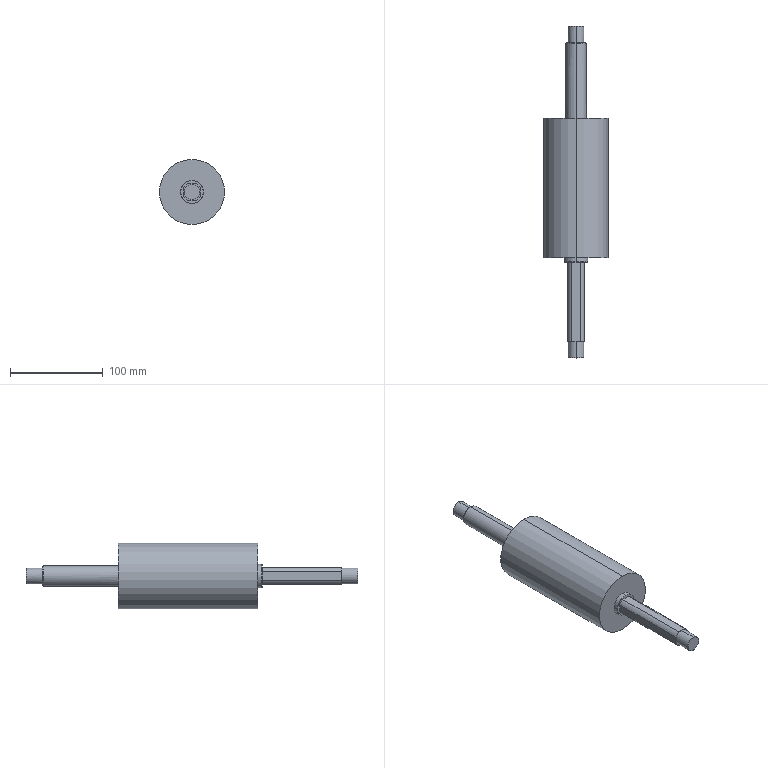Part | STEP file | bevel drive wheel 3_SUS304 | 1 solid | 33 faces | box 70 x 357 x 70 mm | volume 643380 mm3 | cylinder 14 | plane 11 | cone 8 | commonest cylinder face diameters 17 x4 20 x4 22 x2 25 x2 70 x2